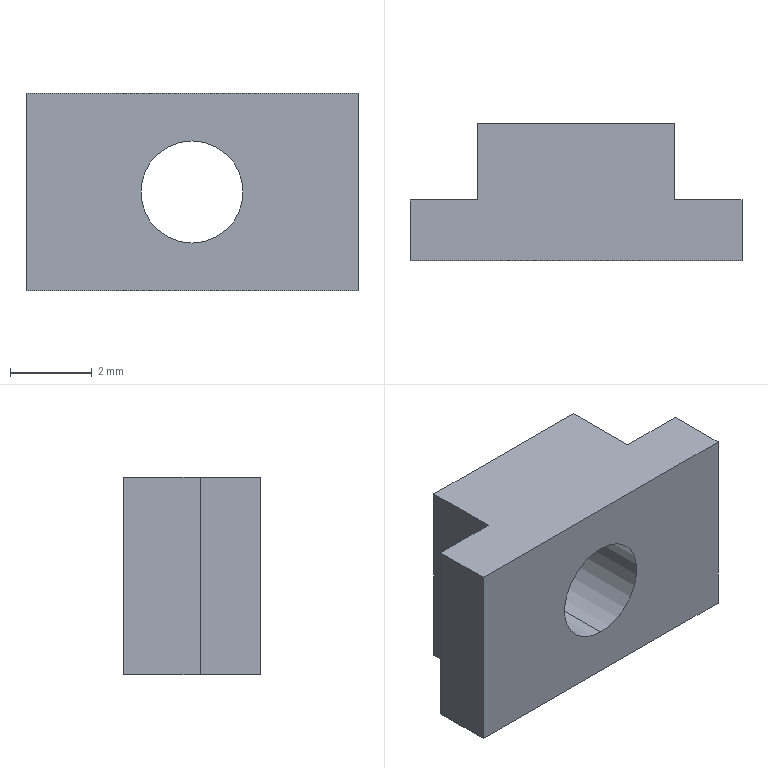Part | NX | features BREP 1 | 1 solid | 12 faces | box 8.13 x 3.36 x 4.83 mm | volume 85.481 mm3 | plane 10 | cylinder 2 | commonest cylinder face diameters 2.5 x2
STEP:
#1=CARTESIAN_POINT('',(0.,0.,1.165));
#2=VERTEX_POINT('',#1);
#3=CARTESIAN_POINT('',(0.,0.,3.665));
#4=VERTEX_POINT('',#3);
#5=CARTESIAN_POINT('',(0.,0.,2.415));
#6=DIRECTION('',(0.,1.,0.));
#7=DIRECTION('',(0.,0.,1.));
#8=AXIS2_PLACEMENT_3D('',#5,#6,#7);
#9=CIRCLE('',#8,1.25);
#10=EDGE_CURVE('',#2,#4,#9,.T.);
#11=ORIENTED_EDGE('',*,*,#10,.F.);
#12=CARTESIAN_POINT('',(0.,3.36,1.165));
#13=VERTEX_POINT('',#12);
#14=CARTESIAN_POINT('',(0.,3.36,1.165));
#15=DIRECTION('',(0.,1.,0.));
#16=VECTOR('',#15,1000.);
#17=LINE('',#14,#16);
#18=EDGE_CURVE('',#13,#2,#17,.F.);
#19=ORIENTED_EDGE('',*,*,#18,.F.);
#20=CARTESIAN_POINT('',(0.,3.36,3.665));
#21=VERTEX_POINT('',#20);
#22=CARTESIAN_POINT('',(0.,3.36,2.415));
#23=DIRECTION('',(0.,1.,0.));
#24=DIRECTION('',(0.,0.,1.));
#25=AXIS2_PLACEMENT_3D('',#22,#23,#24);
#26=CIRCLE('',#25,1.25);
#27=EDGE_CURVE('',#13,#21,#26,.T.);
#28=ORIENTED_EDGE('',*,*,#27,.T.);
#29=CARTESIAN_POINT('',(0.,3.36,3.665));
#30=DIRECTION('',(0.,1.,0.));
#31=VECTOR('',#30,1000.);
#32=LINE('',#29,#31);
#33=EDGE_CURVE('',#21,#4,#32,.F.);
#34=ORIENTED_EDGE('',*,*,#33,.T.);
#35=EDGE_LOOP('',(#11,#19,#28,#34));
#36=FACE_BOUND('',#35,.T.);
#37=CARTESIAN_POINT('',(0.,3.36,2.415));
#38=DIRECTION('',(0.,1.,0.));
#39=DIRECTION('',(0.,0.,1.));
#40=AXIS2_PLACEMENT_3D('',#37,#38,#39);
#41=CYLINDRICAL_SURFACE('',#40,1.25);
#42=ADVANCED_FACE('',(#36),#41,.F.);
#43=CARTESIAN_POINT('',(-4.065,1.48,0.));
#44=VERTEX_POINT('',#43);
#45=CARTESIAN_POINT('',(-4.065,0.,0.));
#46=VERTEX_POINT('',#45);
#47=CARTESIAN_POINT('',(-4.065,0.,0.));
#48=DIRECTION('',(0.,-1.,0.));
#49=VECTOR('',#48,1000.);
#50=LINE('',#47,#49);
#51=EDGE_CURVE('',#44,#46,#50,.T.);
#52=ORIENTED_EDGE('',*,*,#51,.T.);
#53=CARTESIAN_POINT('',(-4.065,0.,4.83));
#54=VERTEX_POINT('',#53);
#55=CARTESIAN_POINT('',(-4.065,0.,4.83));
#56=DIRECTION('',(0.,0.,-1.));
#57=VECTOR('',#56,1000.);
#58=LINE('',#55,#57);
#59=EDGE_CURVE('',#54,#46,#58,.T.);
#60=ORIENTED_EDGE('',*,*,#59,.F.);
#61=CARTESIAN_POINT('',(-4.065,1.48,4.83));
#62=VERTEX_POINT('',#61);
#63=CARTESIAN_POINT('',(-4.065,0.,4.83));
#64=DIRECTION('',(0.,-1.,0.));
#65=VECTOR('',#64,1000.);
#66=LINE('',#63,#65);
#67=EDGE_CURVE('',#62,#54,#66,.T.);
#68=ORIENTED_EDGE('',*,*,#67,.F.);
#69=CARTESIAN_POINT('',(-4.065,1.48,4.83));
#70=DIRECTION('',(0.,0.,-1.));
#71=VECTOR('',#70,1000.);
#72=LINE('',#69,#71);
#73=EDGE_CURVE('',#62,#44,#72,.T.);
#74=ORIENTED_EDGE('',*,*,#73,.T.);
#75=EDGE_LOOP('',(#52,#60,#68,#74));
#76=FACE_BOUND('',#75,.T.);
#77=CARTESIAN_POINT('',(-4.065,0.,4.83));
#78=DIRECTION('',(1.,0.,0.));
#79=DIRECTION('',(0.,1.,0.));
#80=AXIS2_PLACEMENT_3D('',#77,#78,#79);
#81=PLANE('',#80);
#82=ADVANCED_FACE('',(#76),#81,.F.);
#83=CARTESIAN_POINT('',(4.065,0.,0.));
#84=VERTEX_POINT('',#83);
#85=CARTESIAN_POINT('',(-4.065,0.,0.));
#86=DIRECTION('',(1.,0.,0.));
#87=VECTOR('',#86,1000.);
#88=LINE('',#85,#87);
#89=EDGE_CURVE('',#46,#84,#88,.T.);
#90=ORIENTED_EDGE('',*,*,#89,.T.);
#91=CARTESIAN_POINT('',(4.065,0.,4.83));
#92=VERTEX_POINT('',#91);
#93=CARTESIAN_POINT('',(4.065,0.,4.83));
#94=DIRECTION('',(0.,0.,-1.));
#95=VECTOR('',#94,1000.);
#96=LINE('',#93,#95);
#97=EDGE_CURVE('',#92,#84,#96,.T.);
#98=ORIENTED_EDGE('',*,*,#97,.F.);
#99=CARTESIAN_POINT('',(-4.065,0.,4.83));
#100=DIRECTION('',(1.,0.,0.));
#101=VECTOR('',#100,1000.);
#102=LINE('',#99,#101);
#103=EDGE_CURVE('',#54,#92,#102,.T.);
#104=ORIENTED_EDGE('',*,*,#103,.F.);
#105=ORIENTED_EDGE('',*,*,#59,.T.);
#106=EDGE_LOOP('',(#90,#98,#104,#105));
#107=FACE_BOUND('',#106,.T.);
#108=CARTESIAN_POINT('',(0.,0.,2.415));
#109=DIRECTION('',(0.,1.,0.));
#110=DIRECTION('',(0.,0.,1.));
#111=AXIS2_PLACEMENT_3D('',#108,#109,#110);
#112=CIRCLE('',#111,1.25);
#113=EDGE_CURVE('',#4,#2,#112,.T.);
#114=ORIENTED_EDGE('',*,*,#113,.T.);
#115=ORIENTED_EDGE('',*,*,#10,.T.);
#116=EDGE_LOOP('',(#114,#115));
#117=FACE_BOUND('',#116,.T.);
#118=CARTESIAN_POINT('',(-4.065,0.,4.83));
#119=DIRECTION('',(0.,1.,0.));
#120=DIRECTION('',(1.,0.,0.));
#121=AXIS2_PLACEMENT_3D('',#118,#119,#120);
#122=PLANE('',#121);
#123=ADVANCED_FACE('',(#107,#117),#122,.F.);
#124=CARTESIAN_POINT('',(4.065,1.48,0.));
#125=VERTEX_POINT('',#124);
#126=CARTESIAN_POINT('',(4.065,0.,0.));
#127=DIRECTION('',(0.,1.,0.));
#128=VECTOR('',#127,1000.);
#129=LINE('',#126,#128);
#130=EDGE_CURVE('',#84,#125,#129,.T.);
#131=ORIENTED_EDGE('',*,*,#130,.T.);
#132=CARTESIAN_POINT('',(4.065,1.48,4.83));
#133=VERTEX_POINT('',#132);
#134=CARTESIAN_POINT('',(4.065,1.48,4.83));
#135=DIRECTION('',(0.,0.,-1.));
#136=VECTOR('',#135,1000.);
#137=LINE('',#134,#136);
#138=EDGE_CURVE('',#133,#125,#137,.T.);
#139=ORIENTED_EDGE('',*,*,#138,.F.);
#140=CARTESIAN_POINT('',(4.065,0.,4.83));
#141=DIRECTION('',(0.,1.,0.));
#142=VECTOR('',#141,1000.);
#143=LINE('',#140,#142);
#144=EDGE_CURVE('',#92,#133,#143,.T.);
#145=ORIENTED_EDGE('',*,*,#144,.F.);
#146=ORIENTED_EDGE('',*,*,#97,.T.);
#147=EDGE_LOOP('',(#131,#139,#145,#146));
#148=FACE_BOUND('',#147,.T.);
#149=CARTESIAN_POINT('',(4.065,0.,4.83));
#150=DIRECTION('',(-1.,0.,0.));
#151=DIRECTION('',(0.,0.,1.));
#152=AXIS2_PLACEMENT_3D('',#149,#150,#151);
#153=PLANE('',#152);
#154=ADVANCED_FACE('',(#148),#153,.F.);
#155=CARTESIAN_POINT('',(2.415,1.48,0.));
#156=VERTEX_POINT('',#155);
#157=CARTESIAN_POINT('',(2.415,1.48,0.));
#158=DIRECTION('',(-1.,0.,0.));
#159=VECTOR('',#158,1000.);
#160=LINE('',#157,#159);
#161=EDGE_CURVE('',#125,#156,#160,.T.);
#162=ORIENTED_EDGE('',*,*,#161,.T.);
#163=CARTESIAN_POINT('',(2.415,1.48,4.83));
#164=VERTEX_POINT('',#163);
#165=CARTESIAN_POINT('',(2.415,1.48,4.83));
#166=DIRECTION('',(0.,0.,-1.));
#167=VECTOR('',#166,1000.);
#168=LINE('',#165,#167);
#169=EDGE_CURVE('',#164,#156,#168,.T.);
#170=ORIENTED_EDGE('',*,*,#169,.F.);
#171=CARTESIAN_POINT('',(2.415,1.48,4.83));
#172=DIRECTION('',(-1.,0.,0.));
#173=VECTOR('',#172,1000.);
#174=LINE('',#171,#173);
#175=EDGE_CURVE('',#133,#164,#174,.T.);
#176=ORIENTED_EDGE('',*,*,#175,.F.);
#177=ORIENTED_EDGE('',*,*,#138,.T.);
#178=EDGE_LOOP('',(#162,#170,#176,#177));
#179=FACE_BOUND('',#178,.T.);
#180=CARTESIAN_POINT('',(2.415,1.48,4.83));
#181=DIRECTION('',(0.,-1.,0.));
#182=DIRECTION('',(0.,0.,-1.));
#183=AXIS2_PLACEMENT_3D('',#180,#181,#182);
#184=PLANE('',#183);
#185=ADVANCED_FACE('',(#179),#184,.F.);
#186=CARTESIAN_POINT('',(2.415,3.36,0.));
#187=VERTEX_POINT('',#186);
#188=CARTESIAN_POINT('',(2.415,3.36,0.));
#189=DIRECTION('',(0.,1.,0.));
#190=VECTOR('',#189,1000.);
#191=LINE('',#188,#190);
#192=EDGE_CURVE('',#156,#187,#191,.T.);
#193=ORIENTED_EDGE('',*,*,#192,.T.);
#194=CARTESIAN_POINT('',(2.415,3.36,4.83));
#195=VERTEX_POINT('',#194);
#196=CARTESIAN_POINT('',(2.415,3.36,4.83));
#197=DIRECTION('',(0.,0.,-1.));
#198=VECTOR('',#197,1000.);
#199=LINE('',#196,#198);
#200=EDGE_CURVE('',#195,#187,#199,.T.);
#201=ORIENTED_EDGE('',*,*,#200,.F.);
#202=CARTESIAN_POINT('',(2.415,3.36,4.83));
#203=DIRECTION('',(0.,1.,0.));
#204=VECTOR('',#203,1000.);
#205=LINE('',#202,#204);
#206=EDGE_CURVE('',#164,#195,#205,.T.);
#207=ORIENTED_EDGE('',*,*,#206,.F.);
#208=ORIENTED_EDGE('',*,*,#169,.T.);
#209=EDGE_LOOP('',(#193,#201,#207,#208));
#210=FACE_BOUND('',#209,.T.);
#211=CARTESIAN_POINT('',(2.415,3.36,4.83));
#212=DIRECTION('',(-1.,0.,0.));
#213=DIRECTION('',(0.,1.,0.));
#214=AXIS2_PLACEMENT_3D('',#211,#212,#213);
#215=PLANE('',#214);
#216=ADVANCED_FACE('',(#210),#215,.F.);
#217=CARTESIAN_POINT('',(-2.415,3.36,0.));
#218=VERTEX_POINT('',#217);
#219=CARTESIAN_POINT('',(-2.415,3.36,0.));
#220=DIRECTION('',(-1.,0.,0.));
#221=VECTOR('',#220,1000.);
#222=LINE('',#219,#221);
#223=EDGE_CURVE('',#187,#218,#222,.T.);
#224=ORIENTED_EDGE('',*,*,#223,.T.);
#225=CARTESIAN_POINT('',(-2.415,3.36,4.83));
#226=VERTEX_POINT('',#225);
#227=CARTESIAN_POINT('',(-2.415,3.36,4.83));
#228=DIRECTION('',(0.,0.,-1.));
#229=VECTOR('',#228,1000.);
#230=LINE('',#227,#229);
#231=EDGE_CURVE('',#226,#218,#230,.T.);
#232=ORIENTED_EDGE('',*,*,#231,.F.);
#233=CARTESIAN_POINT('',(-2.415,3.36,4.83));
#234=DIRECTION('',(-1.,0.,0.));
#235=VECTOR('',#234,1000.);
#236=LINE('',#233,#235);
#237=EDGE_CURVE('',#195,#226,#236,.T.);
#238=ORIENTED_EDGE('',*,*,#237,.F.);
#239=ORIENTED_EDGE('',*,*,#200,.T.);
#240=EDGE_LOOP('',(#224,#232,#238,#239));
#241=FACE_BOUND('',#240,.T.);
#242=CARTESIAN_POINT('',(0.,3.36,2.415));
#243=DIRECTION('',(0.,1.,0.));
#244=DIRECTION('',(0.,0.,1.));
#245=AXIS2_PLACEMENT_3D('',#242,#243,#244);
#246=CIRCLE('',#245,1.25);
#247=EDGE_CURVE('',#21,#13,#246,.T.);
#248=ORIENTED_EDGE('',*,*,#247,.F.);
#249=ORIENTED_EDGE('',*,*,#27,.F.);
#250=EDGE_LOOP('',(#248,#249));
#251=FACE_BOUND('',#250,.T.);
#252=CARTESIAN_POINT('',(-2.415,3.36,4.83));
#253=DIRECTION('',(0.,-1.,0.));
#254=DIRECTION('',(0.,0.,-1.));
#255=AXIS2_PLACEMENT_3D('',#252,#253,#254);
#256=PLANE('',#255);
#257=ADVANCED_FACE('',(#241,#251),#256,.F.);
#258=CARTESIAN_POINT('',(-2.415,1.48,0.));
#259=VERTEX_POINT('',#258);
#260=CARTESIAN_POINT('',(-2.415,3.36,0.));
#261=DIRECTION('',(0.,-1.,0.));
#262=VECTOR('',#261,1000.);
#263=LINE('',#260,#262);
#264=EDGE_CURVE('',#218,#259,#263,.T.);
#265=ORIENTED_EDGE('',*,*,#264,.T.);
#266=CARTESIAN_POINT('',(-2.415,1.48,4.83));
#267=VERTEX_POINT('',#266);
#268=CARTESIAN_POINT('',(-2.415,1.48,4.83));
#269=DIRECTION('',(0.,0.,-1.));
#270=VECTOR('',#269,1000.);
#271=LINE('',#268,#270);
#272=EDGE_CURVE('',#267,#259,#271,.T.);
#273=ORIENTED_EDGE('',*,*,#272,.F.);
#274=CARTESIAN_POINT('',(-2.415,3.36,4.83));
#275=DIRECTION('',(0.,-1.,0.));
#276=VECTOR('',#275,1000.);
#277=LINE('',#274,#276);
#278=EDGE_CURVE('',#226,#267,#277,.T.);
#279=ORIENTED_EDGE('',*,*,#278,.F.);
#280=ORIENTED_EDGE('',*,*,#231,.T.);
#281=EDGE_LOOP('',(#265,#273,#279,#280));
#282=FACE_BOUND('',#281,.T.);
#283=CARTESIAN_POINT('',(-2.415,3.36,4.83));
#284=DIRECTION('',(1.,0.,0.));
#285=DIRECTION('',(0.,-1.,0.));
#286=AXIS2_PLACEMENT_3D('',#283,#284,#285);
#287=PLANE('',#286);
#288=ADVANCED_FACE('',(#282),#287,.F.);
#289=CARTESIAN_POINT('',(-4.065,1.48,0.));
#290=DIRECTION('',(-1.,0.,0.));
#291=VECTOR('',#290,1000.);
#292=LINE('',#289,#291);
#293=EDGE_CURVE('',#259,#44,#292,.T.);
#294=ORIENTED_EDGE('',*,*,#293,.T.);
#295=ORIENTED_EDGE('',*,*,#73,.F.);
#296=CARTESIAN_POINT('',(-4.065,1.48,4.83));
#297=DIRECTION('',(-1.,0.,0.));
#298=VECTOR('',#297,1000.);
#299=LINE('',#296,#298);
#300=EDGE_CURVE('',#267,#62,#299,.T.);
#301=ORIENTED_EDGE('',*,*,#300,.F.);
#302=ORIENTED_EDGE('',*,*,#272,.T.);
#303=EDGE_LOOP('',(#294,#295,#301,#302));
#304=FACE_BOUND('',#303,.T.);
#305=CARTESIAN_POINT('',(-4.065,1.48,4.83));
#306=DIRECTION('',(0.,-1.,0.));
#307=DIRECTION('',(0.,0.,-1.));
#308=AXIS2_PLACEMENT_3D('',#305,#306,#307);
#309=PLANE('',#308);
#310=ADVANCED_FACE('',(#304),#309,.F.);
#311=ORIENTED_EDGE('',*,*,#67,.T.);
#312=ORIENTED_EDGE('',*,*,#103,.T.);
#313=ORIENTED_EDGE('',*,*,#144,.T.);
#314=ORIENTED_EDGE('',*,*,#175,.T.);
#315=ORIENTED_EDGE('',*,*,#206,.T.);
#316=ORIENTED_EDGE('',*,*,#237,.T.);
#317=ORIENTED_EDGE('',*,*,#278,.T.);
#318=ORIENTED_EDGE('',*,*,#300,.T.);
#319=EDGE_LOOP('',(#311,#312,#313,#314,#315,#316,#317,#318));
#320=FACE_BOUND('',#319,.T.);
#321=CARTESIAN_POINT('',(0.,0.,4.83));
#322=DIRECTION('',(0.,0.,-1.));
#323=DIRECTION('',(0.,-1.,0.));
#324=AXIS2_PLACEMENT_3D('',#321,#322,#323);
#325=PLANE('',#324);
#326=ADVANCED_FACE('',(#320),#325,.F.);
#327=ORIENTED_EDGE('',*,*,#51,.F.);
#328=ORIENTED_EDGE('',*,*,#293,.F.);
#329=ORIENTED_EDGE('',*,*,#264,.F.);
#330=ORIENTED_EDGE('',*,*,#223,.F.);
#331=ORIENTED_EDGE('',*,*,#192,.F.);
#332=ORIENTED_EDGE('',*,*,#161,.F.);
#333=ORIENTED_EDGE('',*,*,#130,.F.);
#334=ORIENTED_EDGE('',*,*,#89,.F.);
#335=EDGE_LOOP('',(#327,#328,#329,#330,#331,#332,#333,#334));
#336=FACE_BOUND('',#335,.T.);
#337=CARTESIAN_POINT('',(0.,0.,0.));
#338=DIRECTION('',(0.,0.,-1.));
#339=DIRECTION('',(0.,-1.,0.));
#340=AXIS2_PLACEMENT_3D('',#337,#338,#339);
#341=PLANE('',#340);
#342=ADVANCED_FACE('',(#336),#341,.T.);
#343=ORIENTED_EDGE('',*,*,#18,.T.);
#344=ORIENTED_EDGE('',*,*,#113,.F.);
#345=ORIENTED_EDGE('',*,*,#33,.F.);
#346=ORIENTED_EDGE('',*,*,#247,.T.);
#347=EDGE_LOOP('',(#343,#344,#345,#346));
#348=FACE_BOUND('',#347,.T.);
#349=CARTESIAN_POINT('',(0.,3.36,2.415));
#350=DIRECTION('',(0.,1.,0.));
#351=DIRECTION('',(0.,0.,1.));
#352=AXIS2_PLACEMENT_3D('',#349,#350,#351);
#353=CYLINDRICAL_SURFACE('',#352,1.25);
#354=ADVANCED_FACE('',(#348),#353,.F.);
#355=CLOSED_SHELL('',(#42,#82,#123,#154,#185,#216,#257,#288,#310,#326,#342,#354));
#356=MANIFOLD_SOLID_BREP('',#355);
#357=(LENGTH_UNIT()NAMED_UNIT(*)SI_UNIT(.MILLI.,.METRE.));
#358=UNCERTAINTY_MEASURE_WITH_UNIT(LENGTH_MEASURE(0.00001),#357,'','');
#359=(NAMED_UNIT(*)PLANE_ANGLE_UNIT()SI_UNIT($,.RADIAN.));
#360=(NAMED_UNIT(*)SI_UNIT($,.STERADIAN.)SOLID_ANGLE_UNIT());
#361=(GEOMETRIC_REPRESENTATION_CONTEXT(3)GLOBAL_UNCERTAINTY_ASSIGNED_CONTEXT((#358))GLOBAL_UNIT_ASSIGNED_CONTEXT((#357,#359,#360))REPRESENTATION_CONTEXT('',''));
#362=ADVANCED_BREP_SHAPE_REPRESENTATION('',(#356),#361);